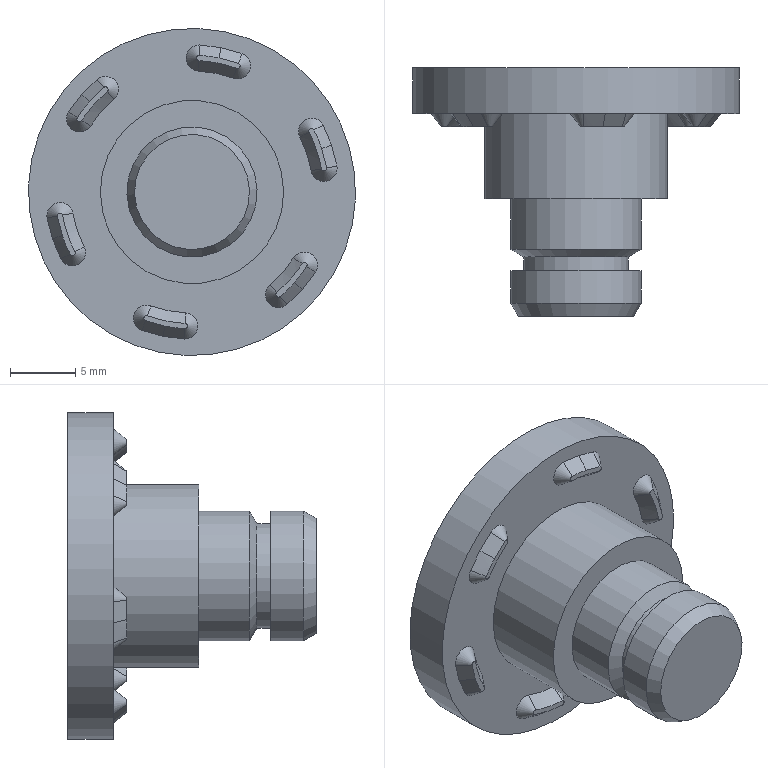Part | STEP file | PRODUTO_PINO | 1 solid | 48 faces | box 25 x 19 x 25 mm | volume 3402 mm3 | spline 30 | plane 11 | cylinder 5 | cone 2 | commonest cylinder face diameters 9.95 x2 8 x1 14 x1 25 x1